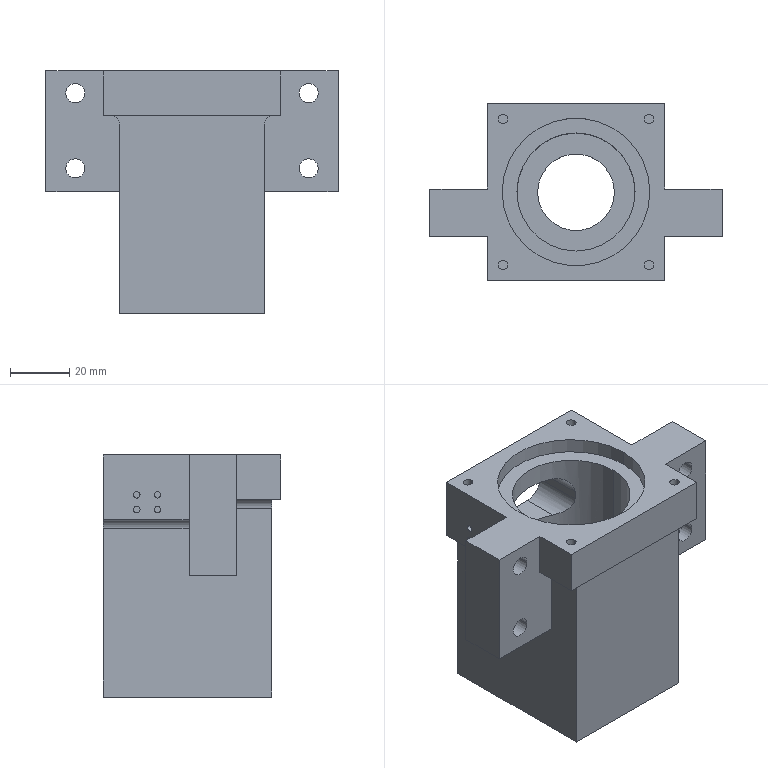Part | STEP file | SM140A-20-1140D-140A-600 Front bearing seat | 1 solid | 122 faces | box 99 x 60 x 82 mm | volume 158063 mm3 | cylinder 68 | plane 52 | cone 2 | commonest cylinder face diameters 2.2 x16 3.2 x16 6.5 x8 11 x8 12 x8 6 x4